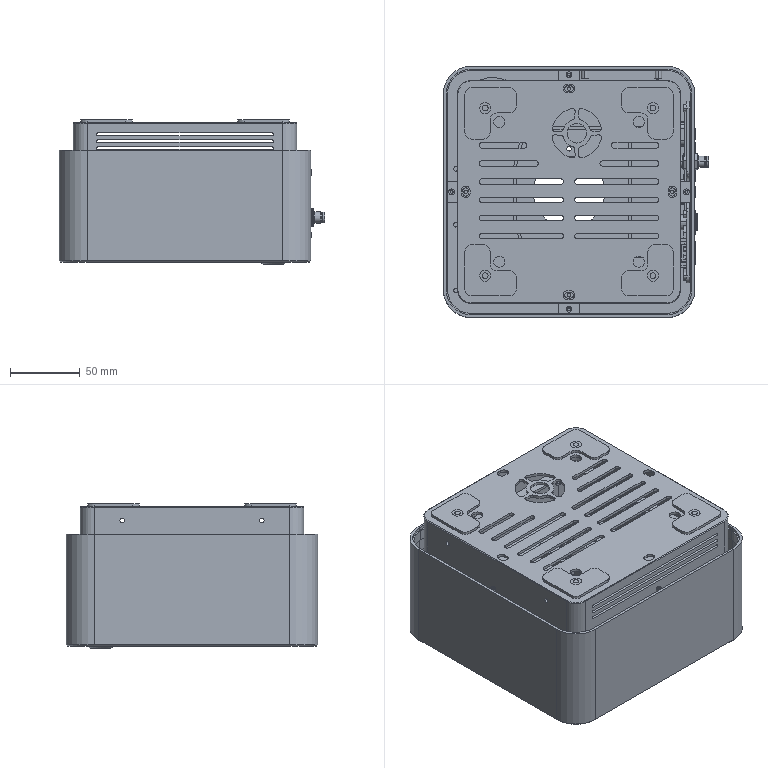Part | NX | features BREP 63 | 64 solids | 3074 faces | volume 318860 mm3 | plane 1578 | cylinder 1043 | spline 323 | cone 104 | torus 18 | sphere 8 | commonest cylinder face diameters 0.2 x155 4 x119 0.6 x80 1 x68 0.4 x59 2.5 x48